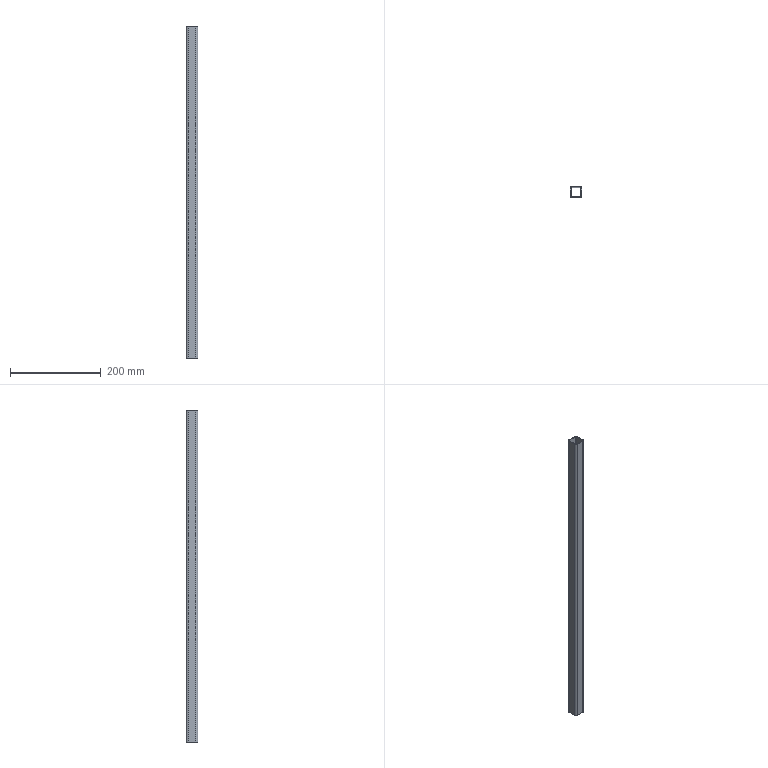Part | SolidWorks | features Extrusion 1 | 1 solid | 18 faces | box 25 x 25 x 730 mm | volume 126800 mm3 | plane 10 | cylinder 8 | commonest cylinder face diameters 4 x4 8 x4
STEP:
#1=CARTESIAN_POINT('',(12.5,8.5,730.));
#2=VERTEX_POINT('',#1);
#3=CARTESIAN_POINT('',(8.5,12.5,730.));
#4=VERTEX_POINT('',#3);
#5=CARTESIAN_POINT('',(8.5,8.5,730.));
#6=DIRECTION('',(0.,0.,1.));
#7=DIRECTION('',(1.,0.,0.));
#8=AXIS2_PLACEMENT_3D('',#5,#6,#7);
#9=CIRCLE('',#8,4.);
#10=EDGE_CURVE('',#2,#4,#9,.T.);
#11=ORIENTED_EDGE('',*,*,#10,.T.);
#12=CARTESIAN_POINT('',(-8.5,12.5,730.));
#13=VERTEX_POINT('',#12);
#14=CARTESIAN_POINT('',(8.5,12.5,730.));
#15=DIRECTION('',(-1.,0.,0.));
#16=VECTOR('',#15,1000.);
#17=LINE('',#14,#16);
#18=EDGE_CURVE('',#4,#13,#17,.T.);
#19=ORIENTED_EDGE('',*,*,#18,.T.);
#20=CARTESIAN_POINT('',(-12.5,8.5,730.));
#21=VERTEX_POINT('',#20);
#22=CARTESIAN_POINT('',(-8.5,8.5,730.));
#23=DIRECTION('',(0.,0.,1.));
#24=DIRECTION('',(1.,0.,0.));
#25=AXIS2_PLACEMENT_3D('',#22,#23,#24);
#26=CIRCLE('',#25,4.);
#27=EDGE_CURVE('',#13,#21,#26,.T.);
#28=ORIENTED_EDGE('',*,*,#27,.T.);
#29=CARTESIAN_POINT('',(-12.5,-8.5,730.));
#30=VERTEX_POINT('',#29);
#31=CARTESIAN_POINT('',(-12.5,-8.5,730.));
#32=DIRECTION('',(0.,-1.,0.));
#33=VECTOR('',#32,1000.);
#34=LINE('',#31,#33);
#35=EDGE_CURVE('',#21,#30,#34,.T.);
#36=ORIENTED_EDGE('',*,*,#35,.T.);
#37=CARTESIAN_POINT('',(-8.5,-12.5,730.));
#38=VERTEX_POINT('',#37);
#39=CARTESIAN_POINT('',(-8.5,-8.5,730.));
#40=DIRECTION('',(0.,0.,1.));
#41=DIRECTION('',(1.,0.,0.));
#42=AXIS2_PLACEMENT_3D('',#39,#40,#41);
#43=CIRCLE('',#42,4.);
#44=EDGE_CURVE('',#30,#38,#43,.T.);
#45=ORIENTED_EDGE('',*,*,#44,.T.);
#46=CARTESIAN_POINT('',(8.5,-12.5,730.));
#47=VERTEX_POINT('',#46);
#48=CARTESIAN_POINT('',(-8.5,-12.5,730.));
#49=DIRECTION('',(1.,0.,0.));
#50=VECTOR('',#49,1000.);
#51=LINE('',#48,#50);
#52=EDGE_CURVE('',#38,#47,#51,.T.);
#53=ORIENTED_EDGE('',*,*,#52,.T.);
#54=CARTESIAN_POINT('',(12.5,-8.5,730.));
#55=VERTEX_POINT('',#54);
#56=CARTESIAN_POINT('',(8.5,-8.5,730.));
#57=DIRECTION('',(0.,0.,1.));
#58=DIRECTION('',(1.,0.,0.));
#59=AXIS2_PLACEMENT_3D('',#56,#57,#58);
#60=CIRCLE('',#59,4.);
#61=EDGE_CURVE('',#47,#55,#60,.T.);
#62=ORIENTED_EDGE('',*,*,#61,.T.);
#63=CARTESIAN_POINT('',(12.5,8.5,730.));
#64=DIRECTION('',(0.,1.,0.));
#65=VECTOR('',#64,1000.);
#66=LINE('',#63,#65);
#67=EDGE_CURVE('',#55,#2,#66,.T.);
#68=ORIENTED_EDGE('',*,*,#67,.T.);
#69=EDGE_LOOP('',(#11,#19,#28,#36,#45,#53,#62,#68));
#70=FACE_OUTER_BOUND('',#69,.T.);
#71=CARTESIAN_POINT('',(-10.5,8.5,730.));
#72=VERTEX_POINT('',#71);
#73=CARTESIAN_POINT('',(-10.5,-8.5,730.));
#74=VERTEX_POINT('',#73);
#75=CARTESIAN_POINT('',(-10.5,-8.5,730.));
#76=DIRECTION('',(0.,-1.,0.));
#77=VECTOR('',#76,1000.);
#78=LINE('',#75,#77);
#79=EDGE_CURVE('',#72,#74,#78,.T.);
#80=ORIENTED_EDGE('',*,*,#79,.F.);
#81=CARTESIAN_POINT('',(-8.5,10.5,730.));
#82=VERTEX_POINT('',#81);
#83=CARTESIAN_POINT('',(-8.5,8.5,730.));
#84=DIRECTION('',(0.,0.,1.));
#85=DIRECTION('',(1.,0.,0.));
#86=AXIS2_PLACEMENT_3D('',#83,#84,#85);
#87=CIRCLE('',#86,2.);
#88=EDGE_CURVE('',#82,#72,#87,.T.);
#89=ORIENTED_EDGE('',*,*,#88,.F.);
#90=CARTESIAN_POINT('',(8.5,10.5,730.));
#91=VERTEX_POINT('',#90);
#92=CARTESIAN_POINT('',(8.5,10.5,730.));
#93=DIRECTION('',(-1.,0.,0.));
#94=VECTOR('',#93,1000.);
#95=LINE('',#92,#94);
#96=EDGE_CURVE('',#91,#82,#95,.T.);
#97=ORIENTED_EDGE('',*,*,#96,.F.);
#98=CARTESIAN_POINT('',(10.5,8.5,730.));
#99=VERTEX_POINT('',#98);
#100=CARTESIAN_POINT('',(8.5,8.5,730.));
#101=DIRECTION('',(0.,0.,1.));
#102=DIRECTION('',(1.,0.,0.));
#103=AXIS2_PLACEMENT_3D('',#100,#101,#102);
#104=CIRCLE('',#103,2.);
#105=EDGE_CURVE('',#99,#91,#104,.T.);
#106=ORIENTED_EDGE('',*,*,#105,.F.);
#107=CARTESIAN_POINT('',(10.5,-8.5,730.));
#108=VERTEX_POINT('',#107);
#109=CARTESIAN_POINT('',(10.5,8.5,730.));
#110=DIRECTION('',(0.,1.,0.));
#111=VECTOR('',#110,1000.);
#112=LINE('',#109,#111);
#113=EDGE_CURVE('',#108,#99,#112,.T.);
#114=ORIENTED_EDGE('',*,*,#113,.F.);
#115=CARTESIAN_POINT('',(8.5,-10.5,730.));
#116=VERTEX_POINT('',#115);
#117=CARTESIAN_POINT('',(8.5,-8.5,730.));
#118=DIRECTION('',(0.,0.,1.));
#119=DIRECTION('',(1.,0.,0.));
#120=AXIS2_PLACEMENT_3D('',#117,#118,#119);
#121=CIRCLE('',#120,2.);
#122=EDGE_CURVE('',#116,#108,#121,.T.);
#123=ORIENTED_EDGE('',*,*,#122,.F.);
#124=CARTESIAN_POINT('',(-8.5,-10.5,730.));
#125=VERTEX_POINT('',#124);
#126=CARTESIAN_POINT('',(-8.5,-10.5,730.));
#127=DIRECTION('',(1.,0.,0.));
#128=VECTOR('',#127,1000.);
#129=LINE('',#126,#128);
#130=EDGE_CURVE('',#125,#116,#129,.T.);
#131=ORIENTED_EDGE('',*,*,#130,.F.);
#132=CARTESIAN_POINT('',(-8.5,-8.5,730.));
#133=DIRECTION('',(0.,0.,1.));
#134=DIRECTION('',(1.,0.,0.));
#135=AXIS2_PLACEMENT_3D('',#132,#133,#134);
#136=CIRCLE('',#135,2.);
#137=EDGE_CURVE('',#74,#125,#136,.T.);
#138=ORIENTED_EDGE('',*,*,#137,.F.);
#139=EDGE_LOOP('',(#80,#89,#97,#106,#114,#123,#131,#138));
#140=FACE_BOUND('',#139,.T.);
#141=CARTESIAN_POINT('',(8.5,8.5,730.));
#142=DIRECTION('',(0.,0.,1.));
#143=DIRECTION('',(1.,0.,0.));
#144=AXIS2_PLACEMENT_3D('',#141,#142,#143);
#145=PLANE('',#144);
#146=ADVANCED_FACE('',(#70,#140),#145,.T.);
#147=CARTESIAN_POINT('',(12.5,8.5,0.));
#148=VERTEX_POINT('',#147);
#149=CARTESIAN_POINT('',(8.5,12.5,0.));
#150=VERTEX_POINT('',#149);
#151=CARTESIAN_POINT('',(8.5,8.5,0.));
#152=DIRECTION('',(0.,0.,1.));
#153=DIRECTION('',(1.,0.,0.));
#154=AXIS2_PLACEMENT_3D('',#151,#152,#153);
#155=CIRCLE('',#154,4.);
#156=EDGE_CURVE('',#148,#150,#155,.T.);
#157=ORIENTED_EDGE('',*,*,#156,.F.);
#158=CARTESIAN_POINT('',(12.5,-8.5,0.));
#159=VERTEX_POINT('',#158);
#160=CARTESIAN_POINT('',(12.5,8.5,0.));
#161=DIRECTION('',(0.,1.,0.));
#162=VECTOR('',#161,1000.);
#163=LINE('',#160,#162);
#164=EDGE_CURVE('',#159,#148,#163,.T.);
#165=ORIENTED_EDGE('',*,*,#164,.F.);
#166=CARTESIAN_POINT('',(8.5,-12.5,0.));
#167=VERTEX_POINT('',#166);
#168=CARTESIAN_POINT('',(8.5,-8.5,0.));
#169=DIRECTION('',(0.,0.,1.));
#170=DIRECTION('',(1.,0.,0.));
#171=AXIS2_PLACEMENT_3D('',#168,#169,#170);
#172=CIRCLE('',#171,4.);
#173=EDGE_CURVE('',#167,#159,#172,.T.);
#174=ORIENTED_EDGE('',*,*,#173,.F.);
#175=CARTESIAN_POINT('',(-8.5,-12.5,0.));
#176=VERTEX_POINT('',#175);
#177=CARTESIAN_POINT('',(-8.5,-12.5,0.));
#178=DIRECTION('',(1.,0.,0.));
#179=VECTOR('',#178,1000.);
#180=LINE('',#177,#179);
#181=EDGE_CURVE('',#176,#167,#180,.T.);
#182=ORIENTED_EDGE('',*,*,#181,.F.);
#183=CARTESIAN_POINT('',(-12.5,-8.5,0.));
#184=VERTEX_POINT('',#183);
#185=CARTESIAN_POINT('',(-8.5,-8.5,0.));
#186=DIRECTION('',(0.,0.,1.));
#187=DIRECTION('',(1.,0.,0.));
#188=AXIS2_PLACEMENT_3D('',#185,#186,#187);
#189=CIRCLE('',#188,4.);
#190=EDGE_CURVE('',#184,#176,#189,.T.);
#191=ORIENTED_EDGE('',*,*,#190,.F.);
#192=CARTESIAN_POINT('',(-12.5,8.5,0.));
#193=VERTEX_POINT('',#192);
#194=CARTESIAN_POINT('',(-12.5,-8.5,0.));
#195=DIRECTION('',(0.,-1.,0.));
#196=VECTOR('',#195,1000.);
#197=LINE('',#194,#196);
#198=EDGE_CURVE('',#193,#184,#197,.T.);
#199=ORIENTED_EDGE('',*,*,#198,.F.);
#200=CARTESIAN_POINT('',(-8.5,12.5,0.));
#201=VERTEX_POINT('',#200);
#202=CARTESIAN_POINT('',(-8.5,8.5,0.));
#203=DIRECTION('',(0.,0.,1.));
#204=DIRECTION('',(1.,0.,0.));
#205=AXIS2_PLACEMENT_3D('',#202,#203,#204);
#206=CIRCLE('',#205,4.);
#207=EDGE_CURVE('',#201,#193,#206,.T.);
#208=ORIENTED_EDGE('',*,*,#207,.F.);
#209=CARTESIAN_POINT('',(8.5,12.5,0.));
#210=DIRECTION('',(-1.,0.,0.));
#211=VECTOR('',#210,1000.);
#212=LINE('',#209,#211);
#213=EDGE_CURVE('',#150,#201,#212,.T.);
#214=ORIENTED_EDGE('',*,*,#213,.F.);
#215=EDGE_LOOP('',(#157,#165,#174,#182,#191,#199,#208,#214));
#216=FACE_OUTER_BOUND('',#215,.T.);
#217=CARTESIAN_POINT('',(-8.5,10.5,0.));
#218=VERTEX_POINT('',#217);
#219=CARTESIAN_POINT('',(-10.5,8.5,0.));
#220=VERTEX_POINT('',#219);
#221=CARTESIAN_POINT('',(-8.5,8.5,0.));
#222=DIRECTION('',(0.,0.,1.));
#223=DIRECTION('',(1.,0.,0.));
#224=AXIS2_PLACEMENT_3D('',#221,#222,#223);
#225=CIRCLE('',#224,2.);
#226=EDGE_CURVE('',#218,#220,#225,.T.);
#227=ORIENTED_EDGE('',*,*,#226,.T.);
#228=CARTESIAN_POINT('',(-10.5,-8.5,0.));
#229=VERTEX_POINT('',#228);
#230=CARTESIAN_POINT('',(-10.5,-8.5,0.));
#231=DIRECTION('',(0.,-1.,0.));
#232=VECTOR('',#231,1000.);
#233=LINE('',#230,#232);
#234=EDGE_CURVE('',#220,#229,#233,.T.);
#235=ORIENTED_EDGE('',*,*,#234,.T.);
#236=CARTESIAN_POINT('',(-8.5,-10.5,0.));
#237=VERTEX_POINT('',#236);
#238=CARTESIAN_POINT('',(-8.5,-8.5,0.));
#239=DIRECTION('',(0.,0.,1.));
#240=DIRECTION('',(1.,0.,0.));
#241=AXIS2_PLACEMENT_3D('',#238,#239,#240);
#242=CIRCLE('',#241,2.);
#243=EDGE_CURVE('',#229,#237,#242,.T.);
#244=ORIENTED_EDGE('',*,*,#243,.T.);
#245=CARTESIAN_POINT('',(8.5,-10.5,0.));
#246=VERTEX_POINT('',#245);
#247=CARTESIAN_POINT('',(-8.5,-10.5,0.));
#248=DIRECTION('',(1.,0.,0.));
#249=VECTOR('',#248,1000.);
#250=LINE('',#247,#249);
#251=EDGE_CURVE('',#237,#246,#250,.T.);
#252=ORIENTED_EDGE('',*,*,#251,.T.);
#253=CARTESIAN_POINT('',(10.5,-8.5,0.));
#254=VERTEX_POINT('',#253);
#255=CARTESIAN_POINT('',(8.5,-8.5,0.));
#256=DIRECTION('',(0.,0.,1.));
#257=DIRECTION('',(1.,0.,0.));
#258=AXIS2_PLACEMENT_3D('',#255,#256,#257);
#259=CIRCLE('',#258,2.);
#260=EDGE_CURVE('',#246,#254,#259,.T.);
#261=ORIENTED_EDGE('',*,*,#260,.T.);
#262=CARTESIAN_POINT('',(10.5,8.5,0.));
#263=VERTEX_POINT('',#262);
#264=CARTESIAN_POINT('',(10.5,8.5,0.));
#265=DIRECTION('',(0.,1.,0.));
#266=VECTOR('',#265,1000.);
#267=LINE('',#264,#266);
#268=EDGE_CURVE('',#254,#263,#267,.T.);
#269=ORIENTED_EDGE('',*,*,#268,.T.);
#270=CARTESIAN_POINT('',(8.5,10.5,0.));
#271=VERTEX_POINT('',#270);
#272=CARTESIAN_POINT('',(8.5,8.5,0.));
#273=DIRECTION('',(0.,0.,1.));
#274=DIRECTION('',(1.,0.,0.));
#275=AXIS2_PLACEMENT_3D('',#272,#273,#274);
#276=CIRCLE('',#275,2.);
#277=EDGE_CURVE('',#263,#271,#276,.T.);
#278=ORIENTED_EDGE('',*,*,#277,.T.);
#279=CARTESIAN_POINT('',(8.5,10.5,0.));
#280=DIRECTION('',(-1.,0.,0.));
#281=VECTOR('',#280,1000.);
#282=LINE('',#279,#281);
#283=EDGE_CURVE('',#271,#218,#282,.T.);
#284=ORIENTED_EDGE('',*,*,#283,.T.);
#285=EDGE_LOOP('',(#227,#235,#244,#252,#261,#269,#278,#284));
#286=FACE_BOUND('',#285,.T.);
#287=CARTESIAN_POINT('',(8.5,8.5,0.));
#288=DIRECTION('',(0.,0.,1.));
#289=DIRECTION('',(1.,0.,0.));
#290=AXIS2_PLACEMENT_3D('',#287,#288,#289);
#291=PLANE('',#290);
#292=ADVANCED_FACE('',(#216,#286),#291,.F.);
#293=ORIENTED_EDGE('',*,*,#156,.T.);
#294=CARTESIAN_POINT('',(8.5,12.5,730.));
#295=DIRECTION('',(0.,0.,-1.));
#296=VECTOR('',#295,1000.);
#297=LINE('',#294,#296);
#298=EDGE_CURVE('',#4,#150,#297,.T.);
#299=ORIENTED_EDGE('',*,*,#298,.F.);
#300=ORIENTED_EDGE('',*,*,#10,.F.);
#301=CARTESIAN_POINT('',(12.5,8.5,730.));
#302=DIRECTION('',(0.,0.,-1.));
#303=VECTOR('',#302,1000.);
#304=LINE('',#301,#303);
#305=EDGE_CURVE('',#2,#148,#304,.T.);
#306=ORIENTED_EDGE('',*,*,#305,.T.);
#307=EDGE_LOOP('',(#293,#299,#300,#306));
#308=FACE_OUTER_BOUND('',#307,.T.);
#309=CARTESIAN_POINT('',(8.5,8.5,730.));
#310=DIRECTION('',(0.,0.,-1.));
#311=DIRECTION('',(-1.,0.,0.));
#312=AXIS2_PLACEMENT_3D('',#309,#310,#311);
#313=CYLINDRICAL_SURFACE('',#312,4.);
#314=ADVANCED_FACE('',(#308),#313,.T.);
#315=ORIENTED_EDGE('',*,*,#213,.T.);
#316=CARTESIAN_POINT('',(-8.5,12.5,730.));
#317=DIRECTION('',(0.,0.,-1.));
#318=VECTOR('',#317,1000.);
#319=LINE('',#316,#318);
#320=EDGE_CURVE('',#13,#201,#319,.T.);
#321=ORIENTED_EDGE('',*,*,#320,.F.);
#322=ORIENTED_EDGE('',*,*,#18,.F.);
#323=ORIENTED_EDGE('',*,*,#298,.T.);
#324=EDGE_LOOP('',(#315,#321,#322,#323));
#325=FACE_OUTER_BOUND('',#324,.T.);
#326=CARTESIAN_POINT('',(8.5,12.5,730.));
#327=DIRECTION('',(0.,-1.,0.));
#328=DIRECTION('',(0.,0.,-1.));
#329=AXIS2_PLACEMENT_3D('',#326,#327,#328);
#330=PLANE('',#329);
#331=ADVANCED_FACE('',(#325),#330,.F.);
#332=ORIENTED_EDGE('',*,*,#207,.T.);
#333=CARTESIAN_POINT('',(-12.5,8.5,730.));
#334=DIRECTION('',(0.,0.,-1.));
#335=VECTOR('',#334,1000.);
#336=LINE('',#333,#335);
#337=EDGE_CURVE('',#21,#193,#336,.T.);
#338=ORIENTED_EDGE('',*,*,#337,.F.);
#339=ORIENTED_EDGE('',*,*,#27,.F.);
#340=ORIENTED_EDGE('',*,*,#320,.T.);
#341=EDGE_LOOP('',(#332,#338,#339,#340));
#342=FACE_OUTER_BOUND('',#341,.T.);
#343=CARTESIAN_POINT('',(-8.5,8.5,730.));
#344=DIRECTION('',(0.,0.,-1.));
#345=DIRECTION('',(-1.,0.,0.));
#346=AXIS2_PLACEMENT_3D('',#343,#344,#345);
#347=CYLINDRICAL_SURFACE('',#346,4.);
#348=ADVANCED_FACE('',(#342),#347,.T.);
#349=ORIENTED_EDGE('',*,*,#198,.T.);
#350=CARTESIAN_POINT('',(-12.5,-8.5,730.));
#351=DIRECTION('',(0.,0.,-1.));
#352=VECTOR('',#351,1000.);
#353=LINE('',#350,#352);
#354=EDGE_CURVE('',#30,#184,#353,.T.);
#355=ORIENTED_EDGE('',*,*,#354,.F.);
#356=ORIENTED_EDGE('',*,*,#35,.F.);
#357=ORIENTED_EDGE('',*,*,#337,.T.);
#358=EDGE_LOOP('',(#349,#355,#356,#357));
#359=FACE_OUTER_BOUND('',#358,.T.);
#360=CARTESIAN_POINT('',(-12.5,-8.5,730.));
#361=DIRECTION('',(1.,0.,0.));
#362=DIRECTION('',(0.,0.,-1.));
#363=AXIS2_PLACEMENT_3D('',#360,#361,#362);
#364=PLANE('',#363);
#365=ADVANCED_FACE('',(#359),#364,.F.);
#366=ORIENTED_EDGE('',*,*,#190,.T.);
#367=CARTESIAN_POINT('',(-8.5,-12.5,730.));
#368=DIRECTION('',(0.,0.,-1.));
#369=VECTOR('',#368,1000.);
#370=LINE('',#367,#369);
#371=EDGE_CURVE('',#38,#176,#370,.T.);
#372=ORIENTED_EDGE('',*,*,#371,.F.);
#373=ORIENTED_EDGE('',*,*,#44,.F.);
#374=ORIENTED_EDGE('',*,*,#354,.T.);
#375=EDGE_LOOP('',(#366,#372,#373,#374));
#376=FACE_OUTER_BOUND('',#375,.T.);
#377=CARTESIAN_POINT('',(-8.5,-8.5,730.));
#378=DIRECTION('',(0.,0.,-1.));
#379=DIRECTION('',(-1.,0.,0.));
#380=AXIS2_PLACEMENT_3D('',#377,#378,#379);
#381=CYLINDRICAL_SURFACE('',#380,4.);
#382=ADVANCED_FACE('',(#376),#381,.T.);
#383=ORIENTED_EDGE('',*,*,#181,.T.);
#384=CARTESIAN_POINT('',(8.5,-12.5,730.));
#385=DIRECTION('',(0.,0.,-1.));
#386=VECTOR('',#385,1000.);
#387=LINE('',#384,#386);
#388=EDGE_CURVE('',#47,#167,#387,.T.);
#389=ORIENTED_EDGE('',*,*,#388,.F.);
#390=ORIENTED_EDGE('',*,*,#52,.F.);
#391=ORIENTED_EDGE('',*,*,#371,.T.);
#392=EDGE_LOOP('',(#383,#389,#390,#391));
#393=FACE_OUTER_BOUND('',#392,.T.);
#394=CARTESIAN_POINT('',(-8.5,-12.5,730.));
#395=DIRECTION('',(0.,1.,0.));
#396=DIRECTION('',(0.,0.,1.));
#397=AXIS2_PLACEMENT_3D('',#394,#395,#396);
#398=PLANE('',#397);
#399=ADVANCED_FACE('',(#393),#398,.F.);
#400=ORIENTED_EDGE('',*,*,#173,.T.);
#401=CARTESIAN_POINT('',(12.5,-8.5,730.));
#402=DIRECTION('',(0.,0.,-1.));
#403=VECTOR('',#402,1000.);
#404=LINE('',#401,#403);
#405=EDGE_CURVE('',#55,#159,#404,.T.);
#406=ORIENTED_EDGE('',*,*,#405,.F.);
#407=ORIENTED_EDGE('',*,*,#61,.F.);
#408=ORIENTED_EDGE('',*,*,#388,.T.);
#409=EDGE_LOOP('',(#400,#406,#407,#408));
#410=FACE_OUTER_BOUND('',#409,.T.);
#411=CARTESIAN_POINT('',(8.5,-8.5,730.));
#412=DIRECTION('',(0.,0.,-1.));
#413=DIRECTION('',(-1.,0.,0.));
#414=AXIS2_PLACEMENT_3D('',#411,#412,#413);
#415=CYLINDRICAL_SURFACE('',#414,4.);
#416=ADVANCED_FACE('',(#410),#415,.T.);
#417=ORIENTED_EDGE('',*,*,#164,.T.);
#418=ORIENTED_EDGE('',*,*,#305,.F.);
#419=ORIENTED_EDGE('',*,*,#67,.F.);
#420=ORIENTED_EDGE('',*,*,#405,.T.);
#421=EDGE_LOOP('',(#417,#418,#419,#420));
#422=FACE_OUTER_BOUND('',#421,.T.);
#423=CARTESIAN_POINT('',(12.5,8.5,730.));
#424=DIRECTION('',(-1.,0.,0.));
#425=DIRECTION('',(0.,0.,1.));
#426=AXIS2_PLACEMENT_3D('',#423,#424,#425);
#427=PLANE('',#426);
#428=ADVANCED_FACE('',(#422),#427,.F.);
#429=ORIENTED_EDGE('',*,*,#226,.F.);
#430=CARTESIAN_POINT('',(-8.5,10.5,730.));
#431=DIRECTION('',(0.,0.,-1.));
#432=VECTOR('',#431,1000.);
#433=LINE('',#430,#432);
#434=EDGE_CURVE('',#82,#218,#433,.T.);
#435=ORIENTED_EDGE('',*,*,#434,.F.);
#436=ORIENTED_EDGE('',*,*,#88,.T.);
#437=CARTESIAN_POINT('',(-10.5,8.5,730.));
#438=DIRECTION('',(0.,0.,-1.));
#439=VECTOR('',#438,1000.);
#440=LINE('',#437,#439);
#441=EDGE_CURVE('',#72,#220,#440,.T.);
#442=ORIENTED_EDGE('',*,*,#441,.T.);
#443=EDGE_LOOP('',(#429,#435,#436,#442));
#444=FACE_OUTER_BOUND('',#443,.T.);
#445=CARTESIAN_POINT('',(-8.5,8.5,730.));
#446=DIRECTION('',(0.,0.,-1.));
#447=DIRECTION('',(-1.,0.,0.));
#448=AXIS2_PLACEMENT_3D('',#445,#446,#447);
#449=CYLINDRICAL_SURFACE('',#448,2.);
#450=ADVANCED_FACE('',(#444),#449,.F.);
#451=ORIENTED_EDGE('',*,*,#234,.F.);
#452=ORIENTED_EDGE('',*,*,#441,.F.);
#453=ORIENTED_EDGE('',*,*,#79,.T.);
#454=CARTESIAN_POINT('',(-10.5,-8.5,730.));
#455=DIRECTION('',(0.,0.,-1.));
#456=VECTOR('',#455,1000.);
#457=LINE('',#454,#456);
#458=EDGE_CURVE('',#74,#229,#457,.T.);
#459=ORIENTED_EDGE('',*,*,#458,.T.);
#460=EDGE_LOOP('',(#451,#452,#453,#459));
#461=FACE_OUTER_BOUND('',#460,.T.);
#462=CARTESIAN_POINT('',(-10.5,-8.5,730.));
#463=DIRECTION('',(1.,0.,0.));
#464=DIRECTION('',(0.,0.,-1.));
#465=AXIS2_PLACEMENT_3D('',#462,#463,#464);
#466=PLANE('',#465);
#467=ADVANCED_FACE('',(#461),#466,.T.);
#468=ORIENTED_EDGE('',*,*,#243,.F.);
#469=ORIENTED_EDGE('',*,*,#458,.F.);
#470=ORIENTED_EDGE('',*,*,#137,.T.);
#471=CARTESIAN_POINT('',(-8.5,-10.5,730.));
#472=DIRECTION('',(0.,0.,-1.));
#473=VECTOR('',#472,1000.);
#474=LINE('',#471,#473);
#475=EDGE_CURVE('',#125,#237,#474,.T.);
#476=ORIENTED_EDGE('',*,*,#475,.T.);
#477=EDGE_LOOP('',(#468,#469,#470,#476));
#478=FACE_OUTER_BOUND('',#477,.T.);
#479=CARTESIAN_POINT('',(-8.5,-8.5,730.));
#480=DIRECTION('',(0.,0.,-1.));
#481=DIRECTION('',(-1.,0.,0.));
#482=AXIS2_PLACEMENT_3D('',#479,#480,#481);
#483=CYLINDRICAL_SURFACE('',#482,2.);
#484=ADVANCED_FACE('',(#478),#483,.F.);
#485=ORIENTED_EDGE('',*,*,#251,.F.);
#486=ORIENTED_EDGE('',*,*,#475,.F.);
#487=ORIENTED_EDGE('',*,*,#130,.T.);
#488=CARTESIAN_POINT('',(8.5,-10.5,730.));
#489=DIRECTION('',(0.,0.,-1.));
#490=VECTOR('',#489,1000.);
#491=LINE('',#488,#490);
#492=EDGE_CURVE('',#116,#246,#491,.T.);
#493=ORIENTED_EDGE('',*,*,#492,.T.);
#494=EDGE_LOOP('',(#485,#486,#487,#493));
#495=FACE_OUTER_BOUND('',#494,.T.);
#496=CARTESIAN_POINT('',(-8.5,-10.5,730.));
#497=DIRECTION('',(0.,1.,0.));
#498=DIRECTION('',(0.,0.,1.));
#499=AXIS2_PLACEMENT_3D('',#496,#497,#498);
#500=PLANE('',#499);
#501=ADVANCED_FACE('',(#495),#500,.T.);
#502=ORIENTED_EDGE('',*,*,#260,.F.);
#503=ORIENTED_EDGE('',*,*,#492,.F.);
#504=ORIENTED_EDGE('',*,*,#122,.T.);
#505=CARTESIAN_POINT('',(10.5,-8.5,730.));
#506=DIRECTION('',(0.,0.,-1.));
#507=VECTOR('',#506,1000.);
#508=LINE('',#505,#507);
#509=EDGE_CURVE('',#108,#254,#508,.T.);
#510=ORIENTED_EDGE('',*,*,#509,.T.);
#511=EDGE_LOOP('',(#502,#503,#504,#510));
#512=FACE_OUTER_BOUND('',#511,.T.);
#513=CARTESIAN_POINT('',(8.5,-8.5,730.));
#514=DIRECTION('',(0.,0.,-1.));
#515=DIRECTION('',(-1.,0.,0.));
#516=AXIS2_PLACEMENT_3D('',#513,#514,#515);
#517=CYLINDRICAL_SURFACE('',#516,2.);
#518=ADVANCED_FACE('',(#512),#517,.F.);
#519=ORIENTED_EDGE('',*,*,#268,.F.);
#520=ORIENTED_EDGE('',*,*,#509,.F.);
#521=ORIENTED_EDGE('',*,*,#113,.T.);
#522=CARTESIAN_POINT('',(10.5,8.5,730.));
#523=DIRECTION('',(0.,0.,-1.));
#524=VECTOR('',#523,1000.);
#525=LINE('',#522,#524);
#526=EDGE_CURVE('',#99,#263,#525,.T.);
#527=ORIENTED_EDGE('',*,*,#526,.T.);
#528=EDGE_LOOP('',(#519,#520,#521,#527));
#529=FACE_OUTER_BOUND('',#528,.T.);
#530=CARTESIAN_POINT('',(10.5,8.5,730.));
#531=DIRECTION('',(-1.,0.,0.));
#532=DIRECTION('',(0.,0.,1.));
#533=AXIS2_PLACEMENT_3D('',#530,#531,#532);
#534=PLANE('',#533);
#535=ADVANCED_FACE('',(#529),#534,.T.);
#536=ORIENTED_EDGE('',*,*,#277,.F.);
#537=ORIENTED_EDGE('',*,*,#526,.F.);
#538=ORIENTED_EDGE('',*,*,#105,.T.);
#539=CARTESIAN_POINT('',(8.5,10.5,730.));
#540=DIRECTION('',(0.,0.,-1.));
#541=VECTOR('',#540,1000.);
#542=LINE('',#539,#541);
#543=EDGE_CURVE('',#91,#271,#542,.T.);
#544=ORIENTED_EDGE('',*,*,#543,.T.);
#545=EDGE_LOOP('',(#536,#537,#538,#544));
#546=FACE_OUTER_BOUND('',#545,.T.);
#547=CARTESIAN_POINT('',(8.5,8.5,730.));
#548=DIRECTION('',(0.,0.,-1.));
#549=DIRECTION('',(-1.,0.,0.));
#550=AXIS2_PLACEMENT_3D('',#547,#548,#549);
#551=CYLINDRICAL_SURFACE('',#550,2.);
#552=ADVANCED_FACE('',(#546),#551,.F.);
#553=ORIENTED_EDGE('',*,*,#283,.F.);
#554=ORIENTED_EDGE('',*,*,#543,.F.);
#555=ORIENTED_EDGE('',*,*,#96,.T.);
#556=ORIENTED_EDGE('',*,*,#434,.T.);
#557=EDGE_LOOP('',(#553,#554,#555,#556));
#558=FACE_OUTER_BOUND('',#557,.T.);
#559=CARTESIAN_POINT('',(8.5,10.5,730.));
#560=DIRECTION('',(0.,-1.,0.));
#561=DIRECTION('',(0.,0.,-1.));
#562=AXIS2_PLACEMENT_3D('',#559,#560,#561);
#563=PLANE('',#562);
#564=ADVANCED_FACE('',(#558),#563,.T.);
#565=CLOSED_SHELL('',(#146,#292,#314,#331,#348,#365,#382,#399,#416,#428,#450,#467,#484,#501,#518,#535,#552,#564));
#566=MANIFOLD_SOLID_BREP('',#565);
#567=CARTESIAN_POINT('',(0.,0.,0.));
#568=DIRECTION('',(0.,0.,1.));
#569=DIRECTION('',(1.,0.,0.));
#570=AXIS2_PLACEMENT_3D('',#567,#568,#569);
#571=(LENGTH_UNIT()NAMED_UNIT(*)SI_UNIT(.MILLI.,.METRE.));
#572=UNCERTAINTY_MEASURE_WITH_UNIT(LENGTH_MEASURE(0.00001),#571,'','');
#573=(NAMED_UNIT(*)PLANE_ANGLE_UNIT()SI_UNIT($,.RADIAN.));
#574=(NAMED_UNIT(*)SI_UNIT($,.STERADIAN.)SOLID_ANGLE_UNIT());
#575=(GEOMETRIC_REPRESENTATION_CONTEXT(3)GLOBAL_UNCERTAINTY_ASSIGNED_CONTEXT((#572))GLOBAL_UNIT_ASSIGNED_CONTEXT((#571,#573,#574))REPRESENTATION_CONTEXT('',''));
#576=ADVANCED_BREP_SHAPE_REPRESENTATION('',(#566,#570),#575);